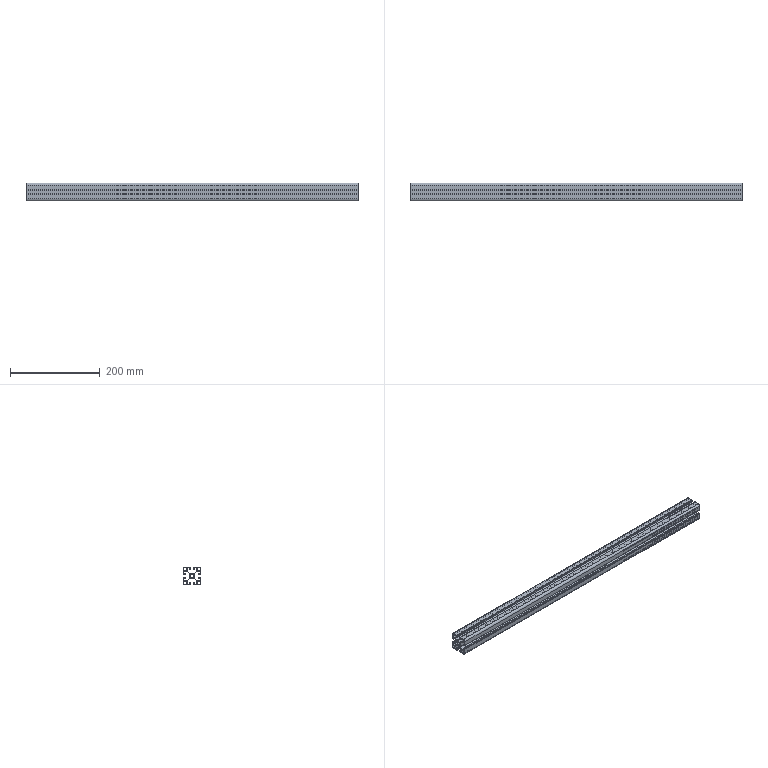Part | STEP file | MK-8-4040C-L-00 Profile 4040C Standard 740mm | 1 solid | 188 faces | box 740 x 40 x 40 mm | volume 353904 mm3 | cylinder 94 | plane 94 | commonest cylinder face diameters 0.6 x30 2 x28 4 x16 0.4 x8 6 x4 9 x4